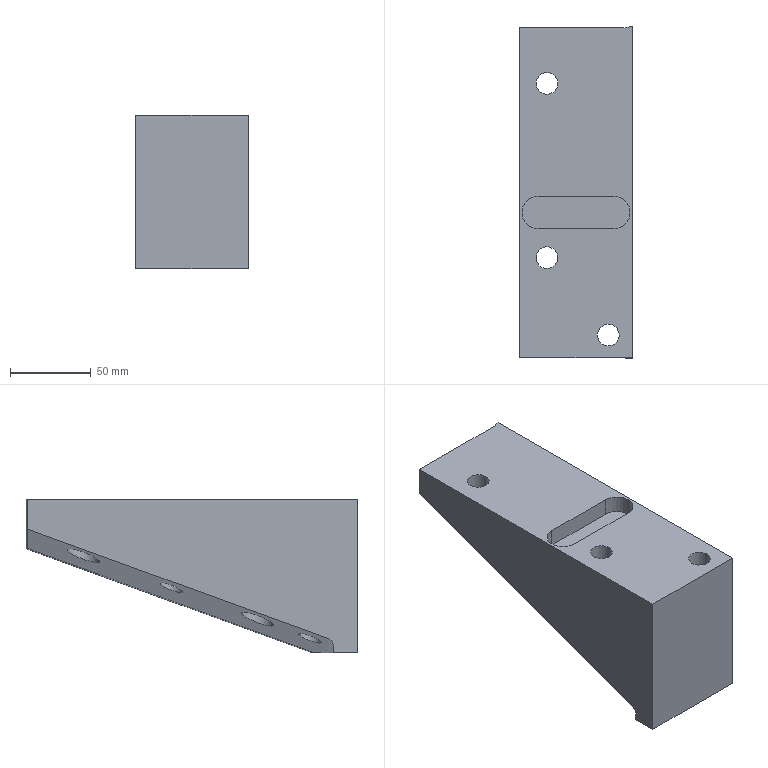Part | STEP file | lll_id3434_x_t | 1 solid | 36 faces | box 70 x 205.551 x 95 mm | volume 826225 mm3 | plane 18 | cylinder 16 | cone 2 | commonest cylinder face diameters 13.509 x3 20 x3 20.008 x3 10.505 x2 14 x2 10 x1
STEP:
#1=CARTESIAN_POINT('',(2591.992,204.547,66.591));
#2=VERTEX_POINT('',#1);
#3=CARTESIAN_POINT('',(2587.172,204.547,67.215));
#4=VERTEX_POINT('',#3);
#5=CARTESIAN_POINT('',(2592.89,204.547,95.841));
#6=DIRECTION('',(0.,1.,0.));
#7=DIRECTION('',(0.000000104,0.,-1.));
#8=AXIS2_PLACEMENT_3D('',#5,#6,#7);
#9=ELLIPSE('',#8,29.265,27.5);
#10=EDGE_CURVE('',#2,#4,#9,.T.);
#11=ORIENTED_EDGE('',*,*,#10,.F.);
#12=CARTESIAN_POINT('',(2592.89,204.547,66.576));
#13=VERTEX_POINT('',#12);
#14=CARTESIAN_POINT('',(2592.89,204.547,95.841));
#15=DIRECTION('',(0.,1.,0.));
#16=DIRECTION('',(0.000000104,0.,-1.));
#17=AXIS2_PLACEMENT_3D('',#14,#15,#16);
#18=ELLIPSE('',#17,29.265,27.5);
#19=EDGE_CURVE('',#13,#2,#18,.T.);
#20=ORIENTED_EDGE('',*,*,#19,.F.);
#21=CARTESIAN_POINT('',(2592.89,30.157,3.103));
#22=VERTEX_POINT('',#21);
#23=CARTESIAN_POINT('',(2592.89,122.985,36.89));
#24=DIRECTION('',(-0.000000036,0.9397,0.342));
#25=VECTOR('',#24,1.);
#26=LINE('',#23,#25);
#27=EDGE_CURVE('',#22,#13,#26,.T.);
#28=ORIENTED_EDGE('',*,*,#27,.F.);
#29=CARTESIAN_POINT('',(2587.172,26.743,2.5));
#30=VERTEX_POINT('',#29);
#31=CARTESIAN_POINT('',(2592.89,30.157,3.103));
#32=CARTESIAN_POINT('',(2590.983,29.077,2.71));
#33=CARTESIAN_POINT('',(2589.064,27.921,2.501));
#34=CARTESIAN_POINT('',(2587.172,26.743,2.5));
#35=B_SPLINE_CURVE_WITH_KNOTS('',3,(#31,#32,#33,#34),.UNSPECIFIED.,.F.,.F.,(4,4),(0.,1.),.UNSPECIFIED.);
#36=EDGE_CURVE('',#22,#30,#35,.T.);
#37=ORIENTED_EDGE('',*,*,#36,.T.);
#38=CARTESIAN_POINT('',(2587.172,112.992,33.892));
#39=DIRECTION('',(0.000000036,-0.9397,-0.342));
#40=VECTOR('',#39,1.);
#41=LINE('',#38,#40);
#42=EDGE_CURVE('',#4,#30,#41,.T.);
#43=ORIENTED_EDGE('',*,*,#42,.F.);
#44=EDGE_LOOP('',(#11,#20,#28,#37,#43));
#45=FACE_OUTER_BOUND('',#44,.T.);
#46=CARTESIAN_POINT('',(2592.89,103.792,59.169));
#47=DIRECTION('',(0.000000036,-0.9397,-0.342));
#48=DIRECTION('',(0.,-0.342,0.9397));
#49=AXIS2_PLACEMENT_3D('',#46,#47,#48);
#50=CYLINDRICAL_SURFACE('',#49,27.5);
#51=ADVANCED_FACE('',(#45),#50,.T.);
#52=CARTESIAN_POINT('',(2535.,15.,2.5));
#53=VERTEX_POINT('',#52);
#54=CARTESIAN_POINT('',(2535.,15.,6.407));
#55=VERTEX_POINT('',#54);
#56=CARTESIAN_POINT('',(2535.,15.,2.5));
#57=DIRECTION('',(0.,0.,1.));
#58=VECTOR('',#57,1.);
#59=LINE('',#56,#58);
#60=EDGE_CURVE('',#53,#55,#59,.T.);
#61=ORIENTED_EDGE('',*,*,#60,.T.);
#62=CARTESIAN_POINT('',(2552.273,15.,2.5));
#63=VERTEX_POINT('',#62);
#64=CARTESIAN_POINT('',(2567.498,15.,-0.9437));
#65=DIRECTION('',(0.9754,0.,-0.2206));
#66=VECTOR('',#65,1.);
#67=LINE('',#64,#66);
#68=EDGE_CURVE('',#55,#63,#67,.T.);
#69=ORIENTED_EDGE('',*,*,#68,.T.);
#70=CARTESIAN_POINT('',(2387.89,15.,2.5));
#71=DIRECTION('',(1.,0.,0.));
#72=VECTOR('',#71,1.);
#73=LINE('',#70,#72);
#74=EDGE_CURVE('',#53,#63,#73,.T.);
#75=ORIENTED_EDGE('',*,*,#74,.F.);
#76=EDGE_LOOP('',(#61,#69,#75));
#77=FACE_OUTER_BOUND('',#76,.T.);
#78=CARTESIAN_POINT('',(2387.89,15.,2.5));
#79=DIRECTION('',(0.,-1.,0.));
#80=DIRECTION('',(1.,0.,0.));
#81=AXIS2_PLACEMENT_3D('',#78,#79,#80);
#82=PLANE('',#81);
#83=ADVANCED_FACE('',(#77),#82,.F.);
#84=CARTESIAN_POINT('',(2535.,18.327,11.238));
#85=VERTEX_POINT('',#84);
#86=CARTESIAN_POINT('',(2535.,20.,6.407));
#87=DIRECTION('',(1.,0.,0.));
#88=DIRECTION('',(0.,0.,1.));
#89=AXIS2_PLACEMENT_3D('',#86,#87,#88);
#90=ELLIPSE('',#89,5.126,5.);
#91=EDGE_CURVE('',#85,#55,#90,.T.);
#92=ORIENTED_EDGE('',*,*,#91,.F.);
#93=CARTESIAN_POINT('',(2573.631,18.327,2.5));
#94=VERTEX_POINT('',#93);
#95=CARTESIAN_POINT('',(2535.261,18.327,11.179));
#96=DIRECTION('',(-0.9754,0.,0.2206));
#97=VECTOR('',#96,1.);
#98=LINE('',#95,#97);
#99=EDGE_CURVE('',#94,#85,#98,.T.);
#100=ORIENTED_EDGE('',*,*,#99,.F.);
#101=CARTESIAN_POINT('',(2552.273,20.,2.5));
#102=DIRECTION('',(0.,0.,1.));
#103=DIRECTION('',(-1.,0.,0.));
#104=AXIS2_PLACEMENT_3D('',#101,#102,#103);
#105=ELLIPSE('',#104,22.663,5.);
#106=EDGE_CURVE('',#63,#94,#105,.T.);
#107=ORIENTED_EDGE('',*,*,#106,.F.);
#108=ORIENTED_EDGE('',*,*,#68,.F.);
#109=EDGE_LOOP('',(#92,#100,#107,#108));
#110=FACE_OUTER_BOUND('',#109,.T.);
#111=CARTESIAN_POINT('',(2395.891,20.,37.873));
#112=DIRECTION('',(-0.9754,0.,0.2206));
#113=DIRECTION('',(-0.2206,0.,-0.9754));
#114=AXIS2_PLACEMENT_3D('',#111,#112,#113);
#115=CYLINDRICAL_SURFACE('',#114,5.);
#116=ADVANCED_FACE('',(#110),#115,.F.);
#117=CARTESIAN_POINT('',(2546.719,70.497,27.575));
#118=VERTEX_POINT('',#117);
#119=CARTESIAN_POINT('',(2552.,62.,23.288));
#120=DIRECTION('',(0.2079,-0.3345,0.9192));
#121=DIRECTION('',(-0.4852,0.7807,0.3939));
#122=AXIS2_PLACEMENT_3D('',#119,#120,#121);
#123=ELLIPSE('',#122,10.884,10.004);
#124=EDGE_CURVE('',#118,#118,#123,.T.);
#125=ORIENTED_EDGE('',*,*,#124,.T.);
#126=EDGE_LOOP('',(#125));
#127=FACE_BOUND('',#126,.T.);
#128=CARTESIAN_POINT('',(2546.719,178.497,66.884));
#129=VERTEX_POINT('',#128);
#130=CARTESIAN_POINT('',(2552.,170.,62.597));
#131=DIRECTION('',(0.2079,-0.3345,0.9192));
#132=DIRECTION('',(-0.4852,0.7807,0.3939));
#133=AXIS2_PLACEMENT_3D('',#130,#131,#132);
#134=ELLIPSE('',#133,10.884,10.004);
#135=EDGE_CURVE('',#129,#129,#134,.T.);
#136=ORIENTED_EDGE('',*,*,#135,.T.);
#137=EDGE_LOOP('',(#136));
#138=FACE_BOUND('',#137,.T.);
#139=CARTESIAN_POINT('',(2548.305,121.445,45.76));
#140=VERTEX_POINT('',#139);
#141=CARTESIAN_POINT('',(2552.,115.5,42.761));
#142=DIRECTION('',(0.2079,-0.3345,0.9192));
#143=DIRECTION('',(-0.4852,0.7807,0.3939));
#144=AXIS2_PLACEMENT_3D('',#141,#142,#143);
#145=ELLIPSE('',#144,7.616,7.);
#146=EDGE_CURVE('',#140,#140,#145,.T.);
#147=ORIENTED_EDGE('',*,*,#146,.T.);
#148=EDGE_LOOP('',(#147));
#149=FACE_BOUND('',#148,.T.);
#150=CARTESIAN_POINT('',(2548.305,35.445,14.459));
#151=VERTEX_POINT('',#150);
#152=CARTESIAN_POINT('',(2552.,29.5,11.459));
#153=DIRECTION('',(0.2079,-0.3345,0.9192));
#154=DIRECTION('',(-0.4852,0.7807,0.3939));
#155=AXIS2_PLACEMENT_3D('',#152,#153,#154);
#156=ELLIPSE('',#155,7.616,7.);
#157=EDGE_CURVE('',#151,#151,#156,.T.);
#158=ORIENTED_EDGE('',*,*,#157,.T.);
#159=EDGE_LOOP('',(#158));
#160=FACE_BOUND('',#159,.T.);
#161=CARTESIAN_POINT('',(2535.,204.547,79.016));
#162=VERTEX_POINT('',#161);
#163=CARTESIAN_POINT('',(2535.,499.68,186.436));
#164=DIRECTION('',(0.,0.9397,0.342));
#165=VECTOR('',#164,1.);
#166=LINE('',#163,#165);
#167=EDGE_CURVE('',#85,#162,#166,.T.);
#168=ORIENTED_EDGE('',*,*,#167,.T.);
#169=CARTESIAN_POINT('',(2555.442,204.547,74.393));
#170=DIRECTION('',(0.9754,0.,-0.2206));
#171=VECTOR('',#170,1.);
#172=LINE('',#169,#171);
#173=EDGE_CURVE('',#162,#4,#172,.T.);
#174=ORIENTED_EDGE('',*,*,#173,.T.);
#175=ORIENTED_EDGE('',*,*,#42,.T.);
#176=CARTESIAN_POINT('',(2587.162,26.737,2.5));
#177=VERTEX_POINT('',#176);
#178=CARTESIAN_POINT('',(4279.499,1078.48,2.5));
#179=DIRECTION('',(0.8493,0.5278,0.));
#180=VECTOR('',#179,1.);
#181=LINE('',#178,#180);
#182=EDGE_CURVE('',#177,#30,#181,.T.);
#183=ORIENTED_EDGE('',*,*,#182,.F.);
#184=CARTESIAN_POINT('',(4279.499,1078.48,2.5));
#185=DIRECTION('',(0.8493,0.5278,0.));
#186=VECTOR('',#185,1.);
#187=LINE('',#184,#186);
#188=EDGE_CURVE('',#94,#177,#187,.T.);
#189=ORIENTED_EDGE('',*,*,#188,.F.);
#190=ORIENTED_EDGE('',*,*,#99,.T.);
#191=EDGE_LOOP('',(#168,#174,#175,#183,#189,#190));
#192=FACE_BOUND('',#191,.T.);
#193=CARTESIAN_POINT('',(2548.048,110.148,41.706));
#194=DIRECTION('',(0.2079,-0.3345,0.9192));
#195=DIRECTION('',(0.,0.9397,0.342));
#196=AXIS2_PLACEMENT_3D('',#193,#194,#195);
#197=PLANE('',#196);
#198=ADVANCED_FACE('',(#127,#138,#149,#160,#192),#197,.F.);
#199=CARTESIAN_POINT('',(2535.,204.547,97.5));
#200=VERTEX_POINT('',#199);
#201=CARTESIAN_POINT('',(2535.,204.547,-1366.758));
#202=DIRECTION('',(0.,0.,1.));
#203=VECTOR('',#202,1.);
#204=LINE('',#201,#203);
#205=EDGE_CURVE('',#162,#200,#204,.T.);
#206=ORIENTED_EDGE('',*,*,#205,.T.);
#207=CARTESIAN_POINT('',(2599.739,204.547,97.5));
#208=VERTEX_POINT('',#207);
#209=CARTESIAN_POINT('',(2418.767,204.547,97.5));
#210=DIRECTION('',(1.,0.,0.));
#211=VECTOR('',#210,1.);
#212=LINE('',#209,#211);
#213=EDGE_CURVE('',#200,#208,#212,.T.);
#214=ORIENTED_EDGE('',*,*,#213,.T.);
#215=CARTESIAN_POINT('',(2599.739,204.547,66.576));
#216=VERTEX_POINT('',#215);
#217=CARTESIAN_POINT('',(2599.739,204.547,-1366.758));
#218=DIRECTION('',(0.,0.,-1.));
#219=VECTOR('',#218,1.);
#220=LINE('',#217,#219);
#221=EDGE_CURVE('',#208,#216,#220,.T.);
#222=ORIENTED_EDGE('',*,*,#221,.T.);
#223=CARTESIAN_POINT('',(2732.617,204.547,66.576));
#224=DIRECTION('',(1.,0.,0.));
#225=VECTOR('',#224,1.);
#226=LINE('',#223,#225);
#227=EDGE_CURVE('',#13,#216,#226,.T.);
#228=ORIENTED_EDGE('',*,*,#227,.F.);
#229=ORIENTED_EDGE('',*,*,#19,.T.);
#230=ORIENTED_EDGE('',*,*,#10,.T.);
#231=ORIENTED_EDGE('',*,*,#173,.F.);
#232=EDGE_LOOP('',(#206,#214,#222,#228,#229,#230,#231));
#233=FACE_OUTER_BOUND('',#232,.T.);
#234=CARTESIAN_POINT('',(2418.767,204.547,-1366.758));
#235=DIRECTION('',(0.,-1.,0.));
#236=DIRECTION('',(0.,0.,1.));
#237=AXIS2_PLACEMENT_3D('',#234,#235,#236);
#238=PLANE('',#237);
#239=ADVANCED_FACE('',(#233),#238,.F.);
#240=ORIENTED_EDGE('',*,*,#221,.F.);
#241=CARTESIAN_POINT('',(2602.331,204.871,97.5));
#242=VERTEX_POINT('',#241);
#243=CARTESIAN_POINT('',(2599.739,215.047,97.5));
#244=DIRECTION('',(0.,0.,-1.));
#245=DIRECTION('',(-1.,0.,0.));
#246=AXIS2_PLACEMENT_3D('',#243,#244,#245);
#247=CIRCLE('',#246,10.5);
#248=EDGE_CURVE('',#242,#208,#247,.T.);
#249=ORIENTED_EDGE('',*,*,#248,.F.);
#250=CARTESIAN_POINT('',(2602.331,204.871,66.694));
#251=VERTEX_POINT('',#250);
#252=CARTESIAN_POINT('',(2602.331,204.871,-74.226));
#253=DIRECTION('',(0.,0.,1.));
#254=VECTOR('',#253,1.);
#255=LINE('',#252,#254);
#256=EDGE_CURVE('',#251,#242,#255,.T.);
#257=ORIENTED_EDGE('',*,*,#256,.F.);
#258=CARTESIAN_POINT('',(2599.739,215.047,70.397));
#259=DIRECTION('',(0.,0.342,-0.9397));
#260=DIRECTION('',(0.,0.9397,0.342));
#261=AXIS2_PLACEMENT_3D('',#258,#259,#260);
#262=ELLIPSE('',#261,11.174,10.5);
#263=EDGE_CURVE('',#251,#216,#262,.T.);
#264=ORIENTED_EDGE('',*,*,#263,.T.);
#265=EDGE_LOOP('',(#240,#249,#257,#264));
#266=FACE_OUTER_BOUND('',#265,.T.);
#267=CARTESIAN_POINT('',(2599.739,215.047,-74.226));
#268=DIRECTION('',(0.,0.,1.));
#269=DIRECTION('',(-1.,0.,0.));
#270=AXIS2_PLACEMENT_3D('',#267,#268,#269);
#271=CYLINDRICAL_SURFACE('',#270,10.5);
#272=ADVANCED_FACE('',(#266),#271,.F.);
#273=CARTESIAN_POINT('',(2605.,205.551,66.941));
#274=VERTEX_POINT('',#273);
#275=CARTESIAN_POINT('',(2605.,205.551,97.5));
#276=VERTEX_POINT('',#275);
#277=CARTESIAN_POINT('',(2605.,205.551,-74.226));
#278=DIRECTION('',(0.,0.,1.));
#279=VECTOR('',#278,1.);
#280=LINE('',#277,#279);
#281=EDGE_CURVE('',#274,#276,#280,.T.);
#282=ORIENTED_EDGE('',*,*,#281,.F.);
#283=CARTESIAN_POINT('',(2701.697,230.18,75.905));
#284=DIRECTION('',(-0.9652,-0.2458,-0.08947));
#285=VECTOR('',#284,1.);
#286=LINE('',#283,#285);
#287=EDGE_CURVE('',#274,#251,#286,.T.);
#288=ORIENTED_EDGE('',*,*,#287,.T.);
#289=ORIENTED_EDGE('',*,*,#256,.T.);
#290=CARTESIAN_POINT('',(2630.962,212.164,97.5));
#291=DIRECTION('',(0.9691,0.2468,0.));
#292=VECTOR('',#291,1.);
#293=LINE('',#290,#292);
#294=EDGE_CURVE('',#242,#276,#293,.T.);
#295=ORIENTED_EDGE('',*,*,#294,.T.);
#296=EDGE_LOOP('',(#282,#288,#289,#295));
#297=FACE_OUTER_BOUND('',#296,.T.);
#298=CARTESIAN_POINT('',(2690.762,227.395,-74.226));
#299=DIRECTION('',(-0.2468,0.9691,0.));
#300=DIRECTION('',(-0.9691,-0.2468,0.));
#301=AXIS2_PLACEMENT_3D('',#298,#299,#300);
#302=PLANE('',#301);
#303=ADVANCED_FACE('',(#297),#302,.T.);
#304=ORIENTED_EDGE('',*,*,#287,.F.);
#305=CARTESIAN_POINT('',(2605.,30.157,3.103));
#306=VERTEX_POINT('',#305);
#307=CARTESIAN_POINT('',(2605.,122.985,36.89));
#308=DIRECTION('',(0.,-0.9397,-0.342));
#309=VECTOR('',#308,1.);
#310=LINE('',#307,#309);
#311=EDGE_CURVE('',#274,#306,#310,.T.);
#312=ORIENTED_EDGE('',*,*,#311,.T.);
#313=CARTESIAN_POINT('',(2732.617,30.157,3.103));
#314=DIRECTION('',(-1.,0.,0.));
#315=VECTOR('',#314,1.);
#316=LINE('',#313,#315);
#317=EDGE_CURVE('',#306,#22,#316,.T.);
#318=ORIENTED_EDGE('',*,*,#317,.T.);
#319=ORIENTED_EDGE('',*,*,#27,.T.);
#320=ORIENTED_EDGE('',*,*,#227,.T.);
#321=ORIENTED_EDGE('',*,*,#263,.F.);
#322=EDGE_LOOP('',(#304,#312,#318,#319,#320,#321));
#323=FACE_OUTER_BOUND('',#322,.T.);
#324=CARTESIAN_POINT('',(2732.617,122.985,36.89));
#325=DIRECTION('',(0.,-0.342,0.9397));
#326=DIRECTION('',(0.,0.9397,0.342));
#327=AXIS2_PLACEMENT_3D('',#324,#325,#326);
#328=PLANE('',#327);
#329=ADVANCED_FACE('',(#323),#328,.F.);
#330=CARTESIAN_POINT('',(2605.,26.737,2.5));
#331=VERTEX_POINT('',#330);
#332=CARTESIAN_POINT('',(2605.,26.737,12.5));
#333=DIRECTION('',(-1.,0.,0.));
#334=DIRECTION('',(0.,0.,1.));
#335=AXIS2_PLACEMENT_3D('',#332,#333,#334);
#336=CIRCLE('',#335,10.);
#337=EDGE_CURVE('',#306,#331,#336,.T.);
#338=ORIENTED_EDGE('',*,*,#337,.T.);
#339=CARTESIAN_POINT('',(13471.883,26.737,2.5));
#340=DIRECTION('',(1.,0.,0.));
#341=VECTOR('',#340,1.);
#342=LINE('',#339,#341);
#343=EDGE_CURVE('',#177,#331,#342,.T.);
#344=ORIENTED_EDGE('',*,*,#343,.F.);
#345=ORIENTED_EDGE('',*,*,#182,.T.);
#346=ORIENTED_EDGE('',*,*,#36,.F.);
#347=ORIENTED_EDGE('',*,*,#317,.F.);
#348=EDGE_LOOP('',(#338,#344,#345,#346,#347));
#349=FACE_OUTER_BOUND('',#348,.T.);
#350=CARTESIAN_POINT('',(13471.883,26.737,12.5));
#351=DIRECTION('',(-1.,0.,0.));
#352=DIRECTION('',(0.,-1.,0.));
#353=AXIS2_PLACEMENT_3D('',#350,#351,#352);
#354=CYLINDRICAL_SURFACE('',#353,10.);
#355=ADVANCED_FACE('',(#349),#354,.T.);
#356=CARTESIAN_POINT('',(2605.,0.00007422,97.5));
#357=VERTEX_POINT('',#356);
#358=CARTESIAN_POINT('',(2605.,0.00007422,97.5));
#359=DIRECTION('',(0.,1.,0.));
#360=VECTOR('',#359,1.);
#361=LINE('',#358,#360);
#362=EDGE_CURVE('',#357,#276,#361,.T.);
#363=ORIENTED_EDGE('',*,*,#362,.F.);
#364=CARTESIAN_POINT('',(2605.,0.00007422,2.5));
#365=VERTEX_POINT('',#364);
#366=CARTESIAN_POINT('',(2605.,0.00007422,52.5));
#367=DIRECTION('',(0.,0.,1.));
#368=VECTOR('',#367,1.);
#369=LINE('',#366,#368);
#370=EDGE_CURVE('',#365,#357,#369,.T.);
#371=ORIENTED_EDGE('',*,*,#370,.F.);
#372=CARTESIAN_POINT('',(2605.,-13712.786,2.5));
#373=DIRECTION('',(0.,1.,0.));
#374=VECTOR('',#373,1.);
#375=LINE('',#372,#374);
#376=EDGE_CURVE('',#365,#331,#375,.T.);
#377=ORIENTED_EDGE('',*,*,#376,.T.);
#378=ORIENTED_EDGE('',*,*,#337,.F.);
#379=ORIENTED_EDGE('',*,*,#311,.F.);
#380=ORIENTED_EDGE('',*,*,#281,.T.);
#381=EDGE_LOOP('',(#363,#371,#377,#378,#379,#380));
#382=FACE_OUTER_BOUND('',#381,.T.);
#383=CARTESIAN_POINT('',(2605.,0.,52.5));
#384=DIRECTION('',(-1.,0.,0.));
#385=DIRECTION('',(0.,0.,1.));
#386=AXIS2_PLACEMENT_3D('',#383,#384,#385);
#387=PLANE('',#386);
#388=ADVANCED_FACE('',(#382),#387,.F.);
#389=CARTESIAN_POINT('',(2593.5,80.,97.5));
#390=VERTEX_POINT('',#389);
#391=CARTESIAN_POINT('',(2546.5,80.,97.5));
#392=VERTEX_POINT('',#391);
#393=CARTESIAN_POINT('',(2685.,80.,97.5));
#394=DIRECTION('',(-1.,0.,0.));
#395=VECTOR('',#394,1.);
#396=LINE('',#393,#395);
#397=EDGE_CURVE('',#390,#392,#396,.T.);
#398=ORIENTED_EDGE('',*,*,#397,.T.);
#399=CARTESIAN_POINT('',(2546.5,100.,97.5));
#400=VERTEX_POINT('',#399);
#401=CARTESIAN_POINT('',(2546.5,90.,97.5));
#402=DIRECTION('',(0.,0.,-1.));
#403=DIRECTION('',(-1.,0.,0.));
#404=AXIS2_PLACEMENT_3D('',#401,#402,#403);
#405=CIRCLE('',#404,10.);
#406=EDGE_CURVE('',#392,#400,#405,.T.);
#407=ORIENTED_EDGE('',*,*,#406,.T.);
#408=CARTESIAN_POINT('',(2593.5,100.,97.5));
#409=VERTEX_POINT('',#408);
#410=CARTESIAN_POINT('',(2685.,100.,97.5));
#411=DIRECTION('',(1.,0.,0.));
#412=VECTOR('',#411,1.);
#413=LINE('',#410,#412);
#414=EDGE_CURVE('',#400,#409,#413,.T.);
#415=ORIENTED_EDGE('',*,*,#414,.T.);
#416=CARTESIAN_POINT('',(2593.5,90.,97.5));
#417=DIRECTION('',(0.,0.,-1.));
#418=DIRECTION('',(-1.,0.,0.));
#419=AXIS2_PLACEMENT_3D('',#416,#417,#418);
#420=CIRCLE('',#419,10.);
#421=EDGE_CURVE('',#409,#390,#420,.T.);
#422=ORIENTED_EDGE('',*,*,#421,.T.);
#423=EDGE_LOOP('',(#398,#407,#415,#422));
#424=FACE_BOUND('',#423,.T.);
#425=CARTESIAN_POINT('',(2545.245,62.,97.5));
#426=VERTEX_POINT('',#425);
#427=CARTESIAN_POINT('',(2552.,62.,97.5));
#428=DIRECTION('',(0.,0.,-1.));
#429=DIRECTION('',(-1.,0.,0.));
#430=AXIS2_PLACEMENT_3D('',#427,#428,#429);
#431=CIRCLE('',#430,6.755);
#432=EDGE_CURVE('',#426,#426,#431,.T.);
#433=ORIENTED_EDGE('',*,*,#432,.T.);
#434=EDGE_LOOP('',(#433));
#435=FACE_BOUND('',#434,.T.);
#436=CARTESIAN_POINT('',(2583.245,14.,97.5));
#437=VERTEX_POINT('',#436);
#438=CARTESIAN_POINT('',(2590.,14.,97.5));
#439=DIRECTION('',(0.,0.,-1.));
#440=DIRECTION('',(-1.,0.,0.));
#441=AXIS2_PLACEMENT_3D('',#438,#439,#440);
#442=CIRCLE('',#441,6.755);
#443=EDGE_CURVE('',#437,#437,#442,.T.);
#444=ORIENTED_EDGE('',*,*,#443,.T.);
#445=EDGE_LOOP('',(#444));
#446=FACE_BOUND('',#445,.T.);
#447=CARTESIAN_POINT('',(2545.245,170.,97.5));
#448=VERTEX_POINT('',#447);
#449=CARTESIAN_POINT('',(2552.,170.,97.5));
#450=DIRECTION('',(0.,0.,-1.));
#451=DIRECTION('',(-1.,0.,0.));
#452=AXIS2_PLACEMENT_3D('',#449,#450,#451);
#453=CIRCLE('',#452,6.755);
#454=EDGE_CURVE('',#448,#448,#453,.T.);
#455=ORIENTED_EDGE('',*,*,#454,.T.);
#456=EDGE_LOOP('',(#455));
#457=FACE_BOUND('',#456,.T.);
#458=CARTESIAN_POINT('',(2535.,0.00007422,97.5));
#459=VERTEX_POINT('',#458);
#460=CARTESIAN_POINT('',(2535.,330.047,97.5));
#461=DIRECTION('',(0.,1.,0.));
#462=VECTOR('',#461,1.);
#463=LINE('',#460,#462);
#464=EDGE_CURVE('',#459,#200,#463,.T.);
#465=ORIENTED_EDGE('',*,*,#464,.F.);
#466=CARTESIAN_POINT('',(2333.342,0.00007422,97.5));
#467=DIRECTION('',(-1.,0.,0.));
#468=VECTOR('',#467,1.);
#469=LINE('',#466,#468);
#470=EDGE_CURVE('',#357,#459,#469,.T.);
#471=ORIENTED_EDGE('',*,*,#470,.F.);
#472=ORIENTED_EDGE('',*,*,#362,.T.);
#473=ORIENTED_EDGE('',*,*,#294,.F.);
#474=ORIENTED_EDGE('',*,*,#248,.T.);
#475=ORIENTED_EDGE('',*,*,#213,.F.);
#476=EDGE_LOOP('',(#465,#471,#472,#473,#474,#475));
#477=FACE_BOUND('',#476,.T.);
#478=CARTESIAN_POINT('',(2685.,0.00007422,97.5));
#479=DIRECTION('',(0.,0.,-1.));
#480=DIRECTION('',(1.,0.,0.));
#481=AXIS2_PLACEMENT_3D('',#478,#479,#480);
#482=PLANE('',#481);
#483=ADVANCED_FACE('',(#424,#435,#446,#457,#477),#482,.F.);
#484=CARTESIAN_POINT('',(2535.,0.00007422,2.5));
#485=VERTEX_POINT('',#484);
#486=CARTESIAN_POINT('',(2535.,330.047,2.5));
#487=DIRECTION('',(0.,1.,0.));
#488=VECTOR('',#487,1.);
#489=LINE('',#486,#488);
#490=EDGE_CURVE('',#485,#53,#489,.T.);
#491=ORIENTED_EDGE('',*,*,#490,.F.);
#492=CARTESIAN_POINT('',(2535.,0.00007422,652.5));
#493=DIRECTION('',(0.,0.,1.));
#494=VECTOR('',#493,1.);
#495=LINE('',#492,#494);
#496=EDGE_CURVE('',#485,#459,#495,.T.);
#497=ORIENTED_EDGE('',*,*,#496,.T.);
#498=ORIENTED_EDGE('',*,*,#464,.T.);
#499=ORIENTED_EDGE('',*,*,#205,.F.);
#500=ORIENTED_EDGE('',*,*,#167,.F.);
#501=ORIENTED_EDGE('',*,*,#91,.T.);
#502=ORIENTED_EDGE('',*,*,#60,.F.);
#503=EDGE_LOOP('',(#491,#497,#498,#499,#500,#501,#502));
#504=FACE_OUTER_BOUND('',#503,.T.);
#505=CARTESIAN_POINT('',(2535.,330.047,652.5));
#506=DIRECTION('',(1.,0.,0.));
#507=DIRECTION('',(0.,0.,1.));
#508=AXIS2_PLACEMENT_3D('',#505,#506,#507);
#509=PLANE('',#508);
#510=ADVANCED_FACE('',(#504),#509,.F.);
#511=CARTESIAN_POINT('',(2579.996,14.,2.5));
#512=VERTEX_POINT('',#511);
#513=CARTESIAN_POINT('',(2590.,14.,2.5));
#514=DIRECTION('',(0.,0.,1.));
#515=DIRECTION('',(-1.,0.,0.));
#516=AXIS2_PLACEMENT_3D('',#513,#514,#515);
#517=CIRCLE('',#516,10.004);
#518=EDGE_CURVE('',#512,#512,#517,.T.);
#519=ORIENTED_EDGE('',*,*,#518,.T.);
#520=EDGE_LOOP('',(#519));
#521=FACE_BOUND('',#520,.T.);
#522=ORIENTED_EDGE('',*,*,#376,.F.);
#523=CARTESIAN_POINT('',(13471.883,0.00007422,2.5));
#524=DIRECTION('',(-1.,0.,0.));
#525=VECTOR('',#524,1.);
#526=LINE('',#523,#525);
#527=EDGE_CURVE('',#365,#485,#526,.T.);
#528=ORIENTED_EDGE('',*,*,#527,.T.);
#529=ORIENTED_EDGE('',*,*,#490,.T.);
#530=ORIENTED_EDGE('',*,*,#74,.T.);
#531=ORIENTED_EDGE('',*,*,#106,.T.);
#532=ORIENTED_EDGE('',*,*,#188,.T.);
#533=ORIENTED_EDGE('',*,*,#343,.T.);
#534=EDGE_LOOP('',(#522,#528,#529,#530,#531,#532,#533));
#535=FACE_BOUND('',#534,.T.);
#536=CARTESIAN_POINT('',(13471.883,-13712.786,2.5));
#537=DIRECTION('',(0.,0.,-1.));
#538=DIRECTION('',(1.,0.,0.));
#539=AXIS2_PLACEMENT_3D('',#536,#537,#538);
#540=PLANE('',#539);
#541=ADVANCED_FACE('',(#521,#535),#540,.T.);
#542=ORIENTED_EDGE('',*,*,#370,.T.);
#543=ORIENTED_EDGE('',*,*,#470,.T.);
#544=ORIENTED_EDGE('',*,*,#496,.F.);
#545=ORIENTED_EDGE('',*,*,#527,.F.);
#546=EDGE_LOOP('',(#542,#543,#544,#545));
#547=FACE_OUTER_BOUND('',#546,.T.);
#548=CARTESIAN_POINT('',(2333.342,0.00007422,1307.5));
#549=DIRECTION('',(0.,1.,0.));
#550=DIRECTION('',(0.,0.,1.));
#551=AXIS2_PLACEMENT_3D('',#548,#549,#550);
#552=PLANE('',#551);
#553=ADVANCED_FACE('',(#547),#552,.F.);
#554=CARTESIAN_POINT('',(2559.,29.5,16.5));
#555=VERTEX_POINT('',#554);
#556=CARTESIAN_POINT('',(2552.,29.5,16.5));
#557=DIRECTION('',(0.,0.,1.));
#558=DIRECTION('',(1.,0.,0.));
#559=AXIS2_PLACEMENT_3D('',#556,#557,#558);
#560=CIRCLE('',#559,7.);
#561=EDGE_CURVE('',#555,#555,#560,.T.);
#562=ORIENTED_EDGE('',*,*,#561,.T.);
#563=EDGE_LOOP('',(#562));
#564=FACE_BOUND('',#563,.T.);
#565=ORIENTED_EDGE('',*,*,#157,.F.);
#566=EDGE_LOOP('',(#565));
#567=FACE_BOUND('',#566,.T.);
#568=CARTESIAN_POINT('',(2552.,29.5,6.5));
#569=DIRECTION('',(0.,0.,1.));
#570=DIRECTION('',(1.,0.,0.));
#571=AXIS2_PLACEMENT_3D('',#568,#569,#570);
#572=CYLINDRICAL_SURFACE('',#571,7.);
#573=ADVANCED_FACE('',(#564,#567),#572,.F.);
#574=CARTESIAN_POINT('',(2557.253,29.5,16.5));
#575=VERTEX_POINT('',#574);
#576=CARTESIAN_POINT('',(2552.,29.5,16.5));
#577=DIRECTION('',(0.,0.,1.));
#578=DIRECTION('',(1.,0.,0.));
#579=AXIS2_PLACEMENT_3D('',#576,#577,#578);
#580=CIRCLE('',#579,5.253);
#581=EDGE_CURVE('',#575,#575,#580,.T.);
#582=ORIENTED_EDGE('',*,*,#581,.T.);
#583=EDGE_LOOP('',(#582));
#584=FACE_BOUND('',#583,.T.);
#585=ORIENTED_EDGE('',*,*,#561,.F.);
#586=EDGE_LOOP('',(#585));
#587=FACE_BOUND('',#586,.T.);
#588=CARTESIAN_POINT('',(2552.,29.5,16.5));
#589=DIRECTION('',(0.,0.,1.));
#590=DIRECTION('',(1.,0.,0.));
#591=AXIS2_PLACEMENT_3D('',#588,#589,#590);
#592=PLANE('',#591);
#593=ADVANCED_FACE('',(#584,#587),#592,.F.);
#594=CARTESIAN_POINT('',(2559.,115.5,48.5));
#595=VERTEX_POINT('',#594);
#596=CARTESIAN_POINT('',(2552.,115.5,48.5));
#597=DIRECTION('',(0.,0.,1.));
#598=DIRECTION('',(1.,0.,0.));
#599=AXIS2_PLACEMENT_3D('',#596,#597,#598);
#600=CIRCLE('',#599,7.);
#601=EDGE_CURVE('',#595,#595,#600,.T.);
#602=ORIENTED_EDGE('',*,*,#601,.T.);
#603=EDGE_LOOP('',(#602));
#604=FACE_BOUND('',#603,.T.);
#605=ORIENTED_EDGE('',*,*,#146,.F.);
#606=EDGE_LOOP('',(#605));
#607=FACE_BOUND('',#606,.T.);
#608=CARTESIAN_POINT('',(2552.,115.5,38.5));
#609=DIRECTION('',(0.,0.,1.));
#610=DIRECTION('',(1.,0.,0.));
#611=AXIS2_PLACEMENT_3D('',#608,#609,#610);
#612=CYLINDRICAL_SURFACE('',#611,7.);
#613=ADVANCED_FACE('',(#604,#607),#612,.F.);
#614=CARTESIAN_POINT('',(2557.253,115.5,48.5));
#615=VERTEX_POINT('',#614);
#616=CARTESIAN_POINT('',(2552.,115.5,48.5));
#617=DIRECTION('',(0.,0.,1.));
#618=DIRECTION('',(1.,0.,0.));
#619=AXIS2_PLACEMENT_3D('',#616,#617,#618);
#620=CIRCLE('',#619,5.253);
#621=EDGE_CURVE('',#615,#615,#620,.T.);
#622=ORIENTED_EDGE('',*,*,#621,.T.);
#623=EDGE_LOOP('',(#622));
#624=FACE_BOUND('',#623,.T.);
#625=ORIENTED_EDGE('',*,*,#601,.F.);
#626=EDGE_LOOP('',(#625));
#627=FACE_BOUND('',#626,.T.);
#628=CARTESIAN_POINT('',(2552.,115.5,48.5));
#629=DIRECTION('',(0.,0.,1.));
#630=DIRECTION('',(1.,0.,0.));
#631=AXIS2_PLACEMENT_3D('',#628,#629,#630);
#632=PLANE('',#631);
#633=ADVANCED_FACE('',(#624,#627),#632,.F.);
#634=CARTESIAN_POINT('',(2557.253,29.5,41.254));
#635=VERTEX_POINT('',#634);
#636=CARTESIAN_POINT('',(2552.,29.5,41.254));
#637=DIRECTION('',(0.,0.,1.));
#638=DIRECTION('',(1.,0.,0.));
#639=AXIS2_PLACEMENT_3D('',#636,#637,#638);
#640=CIRCLE('',#639,5.253);
#641=EDGE_CURVE('',#635,#635,#640,.T.);
#642=ORIENTED_EDGE('',*,*,#641,.T.);
#643=EDGE_LOOP('',(#642));
#644=FACE_BOUND('',#643,.T.);
#645=ORIENTED_EDGE('',*,*,#581,.F.);
#646=EDGE_LOOP('',(#645));
#647=FACE_BOUND('',#646,.T.);
#648=CARTESIAN_POINT('',(2552.,29.5,6.5));
#649=DIRECTION('',(0.,0.,1.));
#650=DIRECTION('',(1.,0.,0.));
#651=AXIS2_PLACEMENT_3D('',#648,#649,#650);
#652=CYLINDRICAL_SURFACE('',#651,5.253);
#653=ADVANCED_FACE('',(#644,#647),#652,.F.);
#654=CARTESIAN_POINT('',(2552.,29.5,46.506));
#655=VERTEX_POINT('',#654);
#656=VERTEX_LOOP('',#655);
#657=FACE_BOUND('',#656,.T.);
#658=ORIENTED_EDGE('',*,*,#641,.F.);
#659=EDGE_LOOP('',(#658));
#660=FACE_BOUND('',#659,.T.);
#661=CARTESIAN_POINT('',(2552.,29.5,41.254));
#662=DIRECTION('',(0.,0.,-1.));
#663=DIRECTION('',(-1.,0.,0.));
#664=AXIS2_PLACEMENT_3D('',#661,#662,#663);
#665=CONICAL_SURFACE('',#664,5.253,45.);
#666=ADVANCED_FACE('',(#657,#660),#665,.F.);
#667=CARTESIAN_POINT('',(2557.253,115.5,73.254));
#668=VERTEX_POINT('',#667);
#669=CARTESIAN_POINT('',(2552.,115.5,73.254));
#670=DIRECTION('',(0.,0.,1.));
#671=DIRECTION('',(1.,0.,0.));
#672=AXIS2_PLACEMENT_3D('',#669,#670,#671);
#673=CIRCLE('',#672,5.253);
#674=EDGE_CURVE('',#668,#668,#673,.T.);
#675=ORIENTED_EDGE('',*,*,#674,.T.);
#676=EDGE_LOOP('',(#675));
#677=FACE_BOUND('',#676,.T.);
#678=ORIENTED_EDGE('',*,*,#621,.F.);
#679=EDGE_LOOP('',(#678));
#680=FACE_BOUND('',#679,.T.);
#681=CARTESIAN_POINT('',(2552.,115.5,38.5));
#682=DIRECTION('',(0.,0.,1.));
#683=DIRECTION('',(1.,0.,0.));
#684=AXIS2_PLACEMENT_3D('',#681,#682,#683);
#685=CYLINDRICAL_SURFACE('',#684,5.253);
#686=ADVANCED_FACE('',(#677,#680),#685,.F.);
#687=CARTESIAN_POINT('',(2552.,115.5,78.506));
#688=VERTEX_POINT('',#687);
#689=VERTEX_LOOP('',#688);
#690=FACE_BOUND('',#689,.T.);
#691=ORIENTED_EDGE('',*,*,#674,.F.);
#692=EDGE_LOOP('',(#691));
#693=FACE_BOUND('',#692,.T.);
#694=CARTESIAN_POINT('',(2552.,115.5,73.254));
#695=DIRECTION('',(0.,0.,-1.));
#696=DIRECTION('',(-1.,0.,0.));
#697=AXIS2_PLACEMENT_3D('',#694,#695,#696);
#698=CONICAL_SURFACE('',#697,5.253,45.);
#699=ADVANCED_FACE('',(#690,#693),#698,.F.);
#700=CARTESIAN_POINT('',(2562.004,170.,81.5));
#701=VERTEX_POINT('',#700);
#702=CARTESIAN_POINT('',(2552.,170.,81.5));
#703=DIRECTION('',(0.,0.,1.));
#704=DIRECTION('',(1.,0.,0.));
#705=AXIS2_PLACEMENT_3D('',#702,#703,#704);
#706=CIRCLE('',#705,10.004);
#707=EDGE_CURVE('',#701,#701,#706,.T.);
#708=ORIENTED_EDGE('',*,*,#707,.T.);
#709=EDGE_LOOP('',(#708));
#710=FACE_BOUND('',#709,.T.);
#711=ORIENTED_EDGE('',*,*,#135,.F.);
#712=EDGE_LOOP('',(#711));
#713=FACE_BOUND('',#712,.T.);
#714=CARTESIAN_POINT('',(2552.,170.,62.5));
#715=DIRECTION('',(0.,0.,1.));
#716=DIRECTION('',(1.,0.,0.));
#717=AXIS2_PLACEMENT_3D('',#714,#715,#716);
#718=CYLINDRICAL_SURFACE('',#717,10.004);
#719=ADVANCED_FACE('',(#710,#713),#718,.F.);
#720=CARTESIAN_POINT('',(2558.755,170.,81.5));
#721=VERTEX_POINT('',#720);
#722=CARTESIAN_POINT('',(2552.,170.,81.5));
#723=DIRECTION('',(0.,0.,1.));
#724=DIRECTION('',(1.,0.,0.));
#725=AXIS2_PLACEMENT_3D('',#722,#723,#724);
#726=CIRCLE('',#725,6.755);
#727=EDGE_CURVE('',#721,#721,#726,.T.);
#728=ORIENTED_EDGE('',*,*,#727,.F.);
#729=EDGE_LOOP('',(#728));
#730=FACE_BOUND('',#729,.T.);
#731=ORIENTED_EDGE('',*,*,#454,.F.);
#732=EDGE_LOOP('',(#731));
#733=FACE_BOUND('',#732,.T.);
#734=CARTESIAN_POINT('',(2552.,170.,62.5));
#735=DIRECTION('',(0.,0.,1.));
#736=DIRECTION('',(1.,0.,0.));
#737=AXIS2_PLACEMENT_3D('',#734,#735,#736);
#738=CYLINDRICAL_SURFACE('',#737,6.755);
#739=ADVANCED_FACE('',(#730,#733),#738,.F.);
#740=ORIENTED_EDGE('',*,*,#727,.T.);
#741=EDGE_LOOP('',(#740));
#742=FACE_BOUND('',#741,.T.);
#743=ORIENTED_EDGE('',*,*,#707,.F.);
#744=EDGE_LOOP('',(#743));
#745=FACE_BOUND('',#744,.T.);
#746=CARTESIAN_POINT('',(2552.,170.,81.5));
#747=DIRECTION('',(0.,0.,1.));
#748=DIRECTION('',(1.,0.,0.));
#749=AXIS2_PLACEMENT_3D('',#746,#747,#748);
#750=PLANE('',#749);
#751=ADVANCED_FACE('',(#742,#745),#750,.F.);
#752=CARTESIAN_POINT('',(2596.755,14.,81.5));
#753=VERTEX_POINT('',#752);
#754=CARTESIAN_POINT('',(2590.,14.,81.5));
#755=DIRECTION('',(0.,0.,1.));
#756=DIRECTION('',(1.,0.,0.));
#757=AXIS2_PLACEMENT_3D('',#754,#755,#756);
#758=CIRCLE('',#757,6.755);
#759=EDGE_CURVE('',#753,#753,#758,.T.);
#760=ORIENTED_EDGE('',*,*,#759,.F.);
#761=EDGE_LOOP('',(#760));
#762=FACE_BOUND('',#761,.T.);
#763=ORIENTED_EDGE('',*,*,#443,.F.);
#764=EDGE_LOOP('',(#763));
#765=FACE_BOUND('',#764,.T.);
#766=CARTESIAN_POINT('',(2590.,14.,62.5));
#767=DIRECTION('',(0.,0.,1.));
#768=DIRECTION('',(1.,0.,0.));
#769=AXIS2_PLACEMENT_3D('',#766,#767,#768);
#770=CYLINDRICAL_SURFACE('',#769,6.755);
#771=ADVANCED_FACE('',(#762,#765),#770,.F.);
#772=CARTESIAN_POINT('',(2600.004,14.,81.5));
#773=VERTEX_POINT('',#772);
#774=CARTESIAN_POINT('',(2590.,14.,81.5));
#775=DIRECTION('',(0.,0.,1.));
#776=DIRECTION('',(1.,0.,0.));
#777=AXIS2_PLACEMENT_3D('',#774,#775,#776);
#778=CIRCLE('',#777,10.004);
#779=EDGE_CURVE('',#773,#773,#778,.T.);
#780=ORIENTED_EDGE('',*,*,#779,.T.);
#781=EDGE_LOOP('',(#780));
#782=FACE_BOUND('',#781,.T.);
#783=ORIENTED_EDGE('',*,*,#518,.F.);
#784=EDGE_LOOP('',(#783));
#785=FACE_BOUND('',#784,.T.);
#786=CARTESIAN_POINT('',(2590.,14.,62.5));
#787=DIRECTION('',(0.,0.,1.));
#788=DIRECTION('',(1.,0.,0.));
#789=AXIS2_PLACEMENT_3D('',#786,#787,#788);
#790=CYLINDRICAL_SURFACE('',#789,10.004);
#791=ADVANCED_FACE('',(#782,#785),#790,.F.);
#792=ORIENTED_EDGE('',*,*,#759,.T.);
#793=EDGE_LOOP('',(#792));
#794=FACE_BOUND('',#793,.T.);
#795=ORIENTED_EDGE('',*,*,#779,.F.);
#796=EDGE_LOOP('',(#795));
#797=FACE_BOUND('',#796,.T.);
#798=CARTESIAN_POINT('',(2552.,170.,81.5));
#799=DIRECTION('',(0.,0.,1.));
#800=DIRECTION('',(1.,0.,0.));
#801=AXIS2_PLACEMENT_3D('',#798,#799,#800);
#802=PLANE('',#801);
#803=ADVANCED_FACE('',(#794,#797),#802,.F.);
#804=CARTESIAN_POINT('',(2562.004,62.,81.5));
#805=VERTEX_POINT('',#804);
#806=CARTESIAN_POINT('',(2552.,62.,81.5));
#807=DIRECTION('',(0.,0.,1.));
#808=DIRECTION('',(1.,0.,0.));
#809=AXIS2_PLACEMENT_3D('',#806,#807,#808);
#810=CIRCLE('',#809,10.004);
#811=EDGE_CURVE('',#805,#805,#810,.T.);
#812=ORIENTED_EDGE('',*,*,#811,.T.);
#813=EDGE_LOOP('',(#812));
#814=FACE_BOUND('',#813,.T.);
#815=ORIENTED_EDGE('',*,*,#124,.F.);
#816=EDGE_LOOP('',(#815));
#817=FACE_BOUND('',#816,.T.);
#818=CARTESIAN_POINT('',(2552.,62.,62.5));
#819=DIRECTION('',(0.,0.,1.));
#820=DIRECTION('',(1.,0.,0.));
#821=AXIS2_PLACEMENT_3D('',#818,#819,#820);
#822=CYLINDRICAL_SURFACE('',#821,10.004);
#823=ADVANCED_FACE('',(#814,#817),#822,.F.);
#824=CARTESIAN_POINT('',(2558.755,62.,81.5));
#825=VERTEX_POINT('',#824);
#826=CARTESIAN_POINT('',(2552.,62.,81.5));
#827=DIRECTION('',(0.,0.,1.));
#828=DIRECTION('',(1.,0.,0.));
#829=AXIS2_PLACEMENT_3D('',#826,#827,#828);
#830=CIRCLE('',#829,6.755);
#831=EDGE_CURVE('',#825,#825,#830,.T.);
#832=ORIENTED_EDGE('',*,*,#831,.F.);
#833=EDGE_LOOP('',(#832));
#834=FACE_BOUND('',#833,.T.);
#835=ORIENTED_EDGE('',*,*,#432,.F.);
#836=EDGE_LOOP('',(#835));
#837=FACE_BOUND('',#836,.T.);
#838=CARTESIAN_POINT('',(2552.,62.,62.5));
#839=DIRECTION('',(0.,0.,1.));
#840=DIRECTION('',(1.,0.,0.));
#841=AXIS2_PLACEMENT_3D('',#838,#839,#840);
#842=CYLINDRICAL_SURFACE('',#841,6.755);
#843=ADVANCED_FACE('',(#834,#837),#842,.F.);
#844=ORIENTED_EDGE('',*,*,#831,.T.);
#845=EDGE_LOOP('',(#844));
#846=FACE_BOUND('',#845,.T.);
#847=ORIENTED_EDGE('',*,*,#811,.F.);
#848=EDGE_LOOP('',(#847));
#849=FACE_BOUND('',#848,.T.);
#850=CARTESIAN_POINT('',(2552.,170.,81.5));
#851=DIRECTION('',(0.,0.,1.));
#852=DIRECTION('',(1.,0.,0.));
#853=AXIS2_PLACEMENT_3D('',#850,#851,#852);
#854=PLANE('',#853);
#855=ADVANCED_FACE('',(#846,#849),#854,.F.);
#856=CARTESIAN_POINT('',(2546.5,100.,86.5));
#857=VERTEX_POINT('',#856);
#858=CARTESIAN_POINT('',(2546.5,100.,107.5));
#859=DIRECTION('',(0.,0.,1.));
#860=VECTOR('',#859,1.);
#861=LINE('',#858,#860);
#862=EDGE_CURVE('',#857,#400,#861,.T.);
#863=ORIENTED_EDGE('',*,*,#862,.F.);
#864=CARTESIAN_POINT('',(2593.5,100.,86.5));
#865=VERTEX_POINT('',#864);
#866=CARTESIAN_POINT('',(2570.,100.,86.5));
#867=DIRECTION('',(-1.,0.,0.));
#868=VECTOR('',#867,1.);
#869=LINE('',#866,#868);
#870=EDGE_CURVE('',#865,#857,#869,.T.);
#871=ORIENTED_EDGE('',*,*,#870,.F.);
#872=CARTESIAN_POINT('',(2593.5,100.,107.5));
#873=DIRECTION('',(0.,0.,-1.));
#874=VECTOR('',#873,1.);
#875=LINE('',#872,#874);
#876=EDGE_CURVE('',#409,#865,#875,.T.);
#877=ORIENTED_EDGE('',*,*,#876,.F.);
#878=ORIENTED_EDGE('',*,*,#414,.F.);
#879=EDGE_LOOP('',(#863,#871,#877,#878));
#880=FACE_OUTER_BOUND('',#879,.T.);
#881=CARTESIAN_POINT('',(2570.,100.,107.5));
#882=DIRECTION('',(0.,1.,0.));
#883=DIRECTION('',(0.,0.,1.));
#884=AXIS2_PLACEMENT_3D('',#881,#882,#883);
#885=PLANE('',#884);
#886=ADVANCED_FACE('',(#880),#885,.F.);
#887=CARTESIAN_POINT('',(2593.5,80.,86.5));
#888=VERTEX_POINT('',#887);
#889=CARTESIAN_POINT('',(2593.5,80.,107.5));
#890=DIRECTION('',(0.,0.,1.));
#891=VECTOR('',#890,1.);
#892=LINE('',#889,#891);
#893=EDGE_CURVE('',#888,#390,#892,.T.);
#894=ORIENTED_EDGE('',*,*,#893,.F.);
#895=CARTESIAN_POINT('',(2546.5,80.,86.5));
#896=VERTEX_POINT('',#895);
#897=CARTESIAN_POINT('',(2570.,80.,86.5));
#898=DIRECTION('',(1.,0.,0.));
#899=VECTOR('',#898,1.);
#900=LINE('',#897,#899);
#901=EDGE_CURVE('',#896,#888,#900,.T.);
#902=ORIENTED_EDGE('',*,*,#901,.F.);
#903=CARTESIAN_POINT('',(2546.5,80.,107.5));
#904=DIRECTION('',(0.,0.,-1.));
#905=VECTOR('',#904,1.);
#906=LINE('',#903,#905);
#907=EDGE_CURVE('',#392,#896,#906,.T.);
#908=ORIENTED_EDGE('',*,*,#907,.F.);
#909=ORIENTED_EDGE('',*,*,#397,.F.);
#910=EDGE_LOOP('',(#894,#902,#908,#909));
#911=FACE_OUTER_BOUND('',#910,.T.);
#912=CARTESIAN_POINT('',(2570.,80.,107.5));
#913=DIRECTION('',(0.,-1.,0.));
#914=DIRECTION('',(0.,0.,-1.));
#915=AXIS2_PLACEMENT_3D('',#912,#913,#914);
#916=PLANE('',#915);
#917=ADVANCED_FACE('',(#911),#916,.F.);
#918=ORIENTED_EDGE('',*,*,#907,.T.);
#919=CARTESIAN_POINT('',(2546.5,90.,86.5));
#920=DIRECTION('',(0.,0.,-1.));
#921=DIRECTION('',(0.,-1.,0.));
#922=AXIS2_PLACEMENT_3D('',#919,#920,#921);
#923=CIRCLE('',#922,10.);
#924=EDGE_CURVE('',#896,#857,#923,.T.);
#925=ORIENTED_EDGE('',*,*,#924,.T.);
#926=ORIENTED_EDGE('',*,*,#862,.T.);
#927=ORIENTED_EDGE('',*,*,#406,.F.);
#928=EDGE_LOOP('',(#918,#925,#926,#927));
#929=FACE_OUTER_BOUND('',#928,.T.);
#930=CARTESIAN_POINT('',(2546.5,90.,107.5));
#931=DIRECTION('',(0.,0.,-1.));
#932=DIRECTION('',(0.,1.,0.));
#933=AXIS2_PLACEMENT_3D('',#930,#931,#932);
#934=CYLINDRICAL_SURFACE('',#933,10.);
#935=ADVANCED_FACE('',(#929),#934,.F.);
#936=ORIENTED_EDGE('',*,*,#876,.T.);
#937=CARTESIAN_POINT('',(2593.5,90.,86.5));
#938=DIRECTION('',(0.,0.,-1.));
#939=DIRECTION('',(0.,-1.,0.));
#940=AXIS2_PLACEMENT_3D('',#937,#938,#939);
#941=CIRCLE('',#940,10.);
#942=EDGE_CURVE('',#865,#888,#941,.T.);
#943=ORIENTED_EDGE('',*,*,#942,.T.);
#944=ORIENTED_EDGE('',*,*,#893,.T.);
#945=ORIENTED_EDGE('',*,*,#421,.F.);
#946=EDGE_LOOP('',(#936,#943,#944,#945));
#947=FACE_OUTER_BOUND('',#946,.T.);
#948=CARTESIAN_POINT('',(2593.5,90.,107.5));
#949=DIRECTION('',(0.,0.,-1.));
#950=DIRECTION('',(0.,1.,0.));
#951=AXIS2_PLACEMENT_3D('',#948,#949,#950);
#952=CYLINDRICAL_SURFACE('',#951,10.);
#953=ADVANCED_FACE('',(#947),#952,.F.);
#954=ORIENTED_EDGE('',*,*,#924,.F.);
#955=ORIENTED_EDGE('',*,*,#901,.T.);
#956=ORIENTED_EDGE('',*,*,#942,.F.);
#957=ORIENTED_EDGE('',*,*,#870,.T.);
#958=EDGE_LOOP('',(#954,#955,#956,#957));
#959=FACE_OUTER_BOUND('',#958,.T.);
#960=CARTESIAN_POINT('',(2570.,90.,86.5));
#961=DIRECTION('',(0.,0.,1.));
#962=DIRECTION('',(0.,-1.,0.));
#963=AXIS2_PLACEMENT_3D('',#960,#961,#962);
#964=PLANE('',#963);
#965=ADVANCED_FACE('',(#959),#964,.T.);
#966=CLOSED_SHELL('',(#51,#83,#116,#198,#239,#272,#303,#329,#355,#388,#483,#510,#541,#553,#573,#593,#613,#633,#653,#666,#686,#699,#719,#739,#751,#771,#791,#803,#823,#843,#855,#886,#917,#935,#953,#965));
#967=MANIFOLD_SOLID_BREP('',#966);
#968=(LENGTH_UNIT()NAMED_UNIT(*)SI_UNIT(.MILLI.,.METRE.));
#969=UNCERTAINTY_MEASURE_WITH_UNIT(LENGTH_MEASURE(0.0508),#968,'','');
#970=(NAMED_UNIT(*)PLANE_ANGLE_UNIT()SI_UNIT($,.RADIAN.));
#971=PLANE_ANGLE_MEASURE_WITH_UNIT(PLANE_ANGLE_MEASURE(0.01745),#970);
#972=DIMENSIONAL_EXPONENTS(0.,0.,0.,0.,0.,0.,0.);
#973=(CONVERSION_BASED_UNIT('DEGREE',#971)NAMED_UNIT(#972)PLANE_ANGLE_UNIT());
#974=(NAMED_UNIT(*)SI_UNIT($,.STERADIAN.)SOLID_ANGLE_UNIT());
#975=(GEOMETRIC_REPRESENTATION_CONTEXT(3)GLOBAL_UNCERTAINTY_ASSIGNED_CONTEXT((#969))GLOBAL_UNIT_ASSIGNED_CONTEXT((#968,#973,#974))REPRESENTATION_CONTEXT('',''));
#976=ADVANCED_BREP_SHAPE_REPRESENTATION('',(#967),#975);